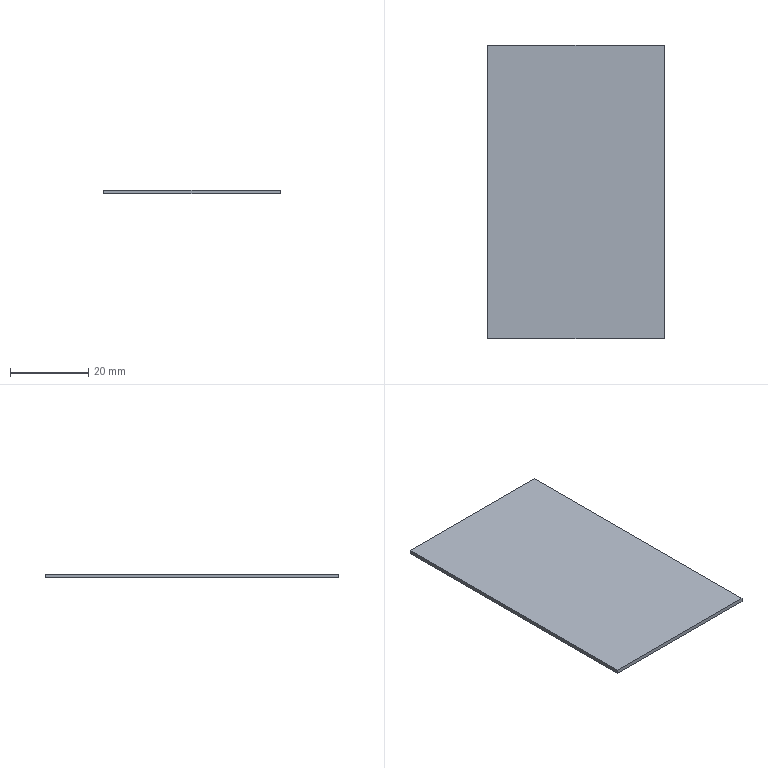Part | STEP file | 7545 cover plate.step.STEP.STEP-323.STEP | 1 solid | 6 faces | box 45 x 75 x 1 mm | volume 3375 mm3 | plane 6
STEP:
#1=CARTESIAN_POINT('',(22.5,-37.5,0.));
#2=VERTEX_POINT('',#1);
#3=CARTESIAN_POINT('',(22.5,37.5,0.));
#4=VERTEX_POINT('',#3);
#5=CARTESIAN_POINT('',(22.5,37.5,0.));
#6=DIRECTION('',(0.,1.,0.));
#7=VECTOR('',#6,1000.);
#8=LINE('',#5,#7);
#9=EDGE_CURVE('',#2,#4,#8,.T.);
#10=ORIENTED_EDGE('',*,*,#9,.T.);
#11=CARTESIAN_POINT('',(22.5,37.5,1.));
#12=VERTEX_POINT('',#11);
#13=CARTESIAN_POINT('',(22.5,37.5,1.));
#14=DIRECTION('',(0.,0.,-1.));
#15=VECTOR('',#14,1000.);
#16=LINE('',#13,#15);
#17=EDGE_CURVE('',#12,#4,#16,.T.);
#18=ORIENTED_EDGE('',*,*,#17,.F.);
#19=CARTESIAN_POINT('',(22.5,-37.5,1.));
#20=VERTEX_POINT('',#19);
#21=CARTESIAN_POINT('',(22.5,37.5,1.));
#22=DIRECTION('',(0.,1.,0.));
#23=VECTOR('',#22,1000.);
#24=LINE('',#21,#23);
#25=EDGE_CURVE('',#20,#12,#24,.T.);
#26=ORIENTED_EDGE('',*,*,#25,.F.);
#27=CARTESIAN_POINT('',(22.5,-37.5,1.));
#28=DIRECTION('',(0.,0.,-1.));
#29=VECTOR('',#28,1000.);
#30=LINE('',#27,#29);
#31=EDGE_CURVE('',#20,#2,#30,.T.);
#32=ORIENTED_EDGE('',*,*,#31,.T.);
#33=EDGE_LOOP('',(#10,#18,#26,#32));
#34=FACE_OUTER_BOUND('',#33,.T.);
#35=CARTESIAN_POINT('',(22.5,37.5,1.));
#36=DIRECTION('',(-1.,0.,0.));
#37=DIRECTION('',(0.,0.,1.));
#38=AXIS2_PLACEMENT_3D('',#35,#36,#37);
#39=PLANE('',#38);
#40=ADVANCED_FACE('',(#34),#39,.F.);
#41=CARTESIAN_POINT('',(-22.5,37.5,0.));
#42=VERTEX_POINT('',#41);
#43=CARTESIAN_POINT('',(-22.5,37.5,0.));
#44=DIRECTION('',(-1.,0.,0.));
#45=VECTOR('',#44,1000.);
#46=LINE('',#43,#45);
#47=EDGE_CURVE('',#4,#42,#46,.T.);
#48=ORIENTED_EDGE('',*,*,#47,.T.);
#49=CARTESIAN_POINT('',(-22.5,37.5,1.));
#50=VERTEX_POINT('',#49);
#51=CARTESIAN_POINT('',(-22.5,37.5,1.));
#52=DIRECTION('',(0.,0.,-1.));
#53=VECTOR('',#52,1000.);
#54=LINE('',#51,#53);
#55=EDGE_CURVE('',#50,#42,#54,.T.);
#56=ORIENTED_EDGE('',*,*,#55,.F.);
#57=CARTESIAN_POINT('',(-22.5,37.5,1.));
#58=DIRECTION('',(-1.,0.,0.));
#59=VECTOR('',#58,1000.);
#60=LINE('',#57,#59);
#61=EDGE_CURVE('',#12,#50,#60,.T.);
#62=ORIENTED_EDGE('',*,*,#61,.F.);
#63=ORIENTED_EDGE('',*,*,#17,.T.);
#64=EDGE_LOOP('',(#48,#56,#62,#63));
#65=FACE_OUTER_BOUND('',#64,.T.);
#66=CARTESIAN_POINT('',(-22.5,37.5,1.));
#67=DIRECTION('',(0.,-1.,0.));
#68=DIRECTION('',(0.,0.,-1.));
#69=AXIS2_PLACEMENT_3D('',#66,#67,#68);
#70=PLANE('',#69);
#71=ADVANCED_FACE('',(#65),#70,.F.);
#72=CARTESIAN_POINT('',(-22.5,-37.5,0.));
#73=VERTEX_POINT('',#72);
#74=CARTESIAN_POINT('',(-22.5,37.5,0.));
#75=DIRECTION('',(0.,-1.,0.));
#76=VECTOR('',#75,1000.);
#77=LINE('',#74,#76);
#78=EDGE_CURVE('',#42,#73,#77,.T.);
#79=ORIENTED_EDGE('',*,*,#78,.T.);
#80=CARTESIAN_POINT('',(-22.5,-37.5,1.));
#81=VERTEX_POINT('',#80);
#82=CARTESIAN_POINT('',(-22.5,-37.5,1.));
#83=DIRECTION('',(0.,0.,-1.));
#84=VECTOR('',#83,1000.);
#85=LINE('',#82,#84);
#86=EDGE_CURVE('',#81,#73,#85,.T.);
#87=ORIENTED_EDGE('',*,*,#86,.F.);
#88=CARTESIAN_POINT('',(-22.5,37.5,1.));
#89=DIRECTION('',(0.,-1.,0.));
#90=VECTOR('',#89,1000.);
#91=LINE('',#88,#90);
#92=EDGE_CURVE('',#50,#81,#91,.T.);
#93=ORIENTED_EDGE('',*,*,#92,.F.);
#94=ORIENTED_EDGE('',*,*,#55,.T.);
#95=EDGE_LOOP('',(#79,#87,#93,#94));
#96=FACE_OUTER_BOUND('',#95,.T.);
#97=CARTESIAN_POINT('',(-22.5,37.5,1.));
#98=DIRECTION('',(1.,0.,0.));
#99=DIRECTION('',(0.,1.,0.));
#100=AXIS2_PLACEMENT_3D('',#97,#98,#99);
#101=PLANE('',#100);
#102=ADVANCED_FACE('',(#96),#101,.F.);
#103=CARTESIAN_POINT('',(-22.5,-37.5,0.));
#104=DIRECTION('',(1.,0.,0.));
#105=VECTOR('',#104,1000.);
#106=LINE('',#103,#105);
#107=EDGE_CURVE('',#73,#2,#106,.T.);
#108=ORIENTED_EDGE('',*,*,#107,.T.);
#109=ORIENTED_EDGE('',*,*,#31,.F.);
#110=CARTESIAN_POINT('',(-22.5,-37.5,1.));
#111=DIRECTION('',(1.,0.,0.));
#112=VECTOR('',#111,1000.);
#113=LINE('',#110,#112);
#114=EDGE_CURVE('',#81,#20,#113,.T.);
#115=ORIENTED_EDGE('',*,*,#114,.F.);
#116=ORIENTED_EDGE('',*,*,#86,.T.);
#117=EDGE_LOOP('',(#108,#109,#115,#116));
#118=FACE_OUTER_BOUND('',#117,.T.);
#119=CARTESIAN_POINT('',(-22.5,-37.5,1.));
#120=DIRECTION('',(0.,1.,0.));
#121=DIRECTION('',(1.,0.,0.));
#122=AXIS2_PLACEMENT_3D('',#119,#120,#121);
#123=PLANE('',#122);
#124=ADVANCED_FACE('',(#118),#123,.F.);
#125=ORIENTED_EDGE('',*,*,#25,.T.);
#126=ORIENTED_EDGE('',*,*,#61,.T.);
#127=ORIENTED_EDGE('',*,*,#92,.T.);
#128=ORIENTED_EDGE('',*,*,#114,.T.);
#129=EDGE_LOOP('',(#125,#126,#127,#128));
#130=FACE_OUTER_BOUND('',#129,.T.);
#131=CARTESIAN_POINT('',(0.,0.,1.));
#132=DIRECTION('',(0.,0.,1.));
#133=DIRECTION('',(1.,0.,0.));
#134=AXIS2_PLACEMENT_3D('',#131,#132,#133);
#135=PLANE('',#134);
#136=ADVANCED_FACE('',(#130),#135,.T.);
#137=ORIENTED_EDGE('',*,*,#9,.F.);
#138=ORIENTED_EDGE('',*,*,#107,.F.);
#139=ORIENTED_EDGE('',*,*,#78,.F.);
#140=ORIENTED_EDGE('',*,*,#47,.F.);
#141=EDGE_LOOP('',(#137,#138,#139,#140));
#142=FACE_OUTER_BOUND('',#141,.T.);
#143=CARTESIAN_POINT('',(0.,0.,0.));
#144=DIRECTION('',(0.,0.,1.));
#145=DIRECTION('',(1.,0.,0.));
#146=AXIS2_PLACEMENT_3D('',#143,#144,#145);
#147=PLANE('',#146);
#148=ADVANCED_FACE('',(#142),#147,.F.);
#149=CLOSED_SHELL('',(#40,#71,#102,#124,#136,#148));
#150=MANIFOLD_SOLID_BREP('',#149);
#151=CARTESIAN_POINT('',(0.,0.,0.));
#152=DIRECTION('',(0.,0.,1.));
#153=DIRECTION('',(1.,0.,0.));
#154=AXIS2_PLACEMENT_3D('',#151,#152,#153);
#155=(LENGTH_UNIT()NAMED_UNIT(*)SI_UNIT(.MILLI.,.METRE.));
#156=UNCERTAINTY_MEASURE_WITH_UNIT(LENGTH_MEASURE(0.00001),#155,'','');
#157=(NAMED_UNIT(*)PLANE_ANGLE_UNIT()SI_UNIT($,.RADIAN.));
#158=(NAMED_UNIT(*)SI_UNIT($,.STERADIAN.)SOLID_ANGLE_UNIT());
#159=(GEOMETRIC_REPRESENTATION_CONTEXT(3)GLOBAL_UNCERTAINTY_ASSIGNED_CONTEXT((#156))GLOBAL_UNIT_ASSIGNED_CONTEXT((#155,#157,#158))REPRESENTATION_CONTEXT('',''));
#160=ADVANCED_BREP_SHAPE_REPRESENTATION('',(#150,#154),#159);